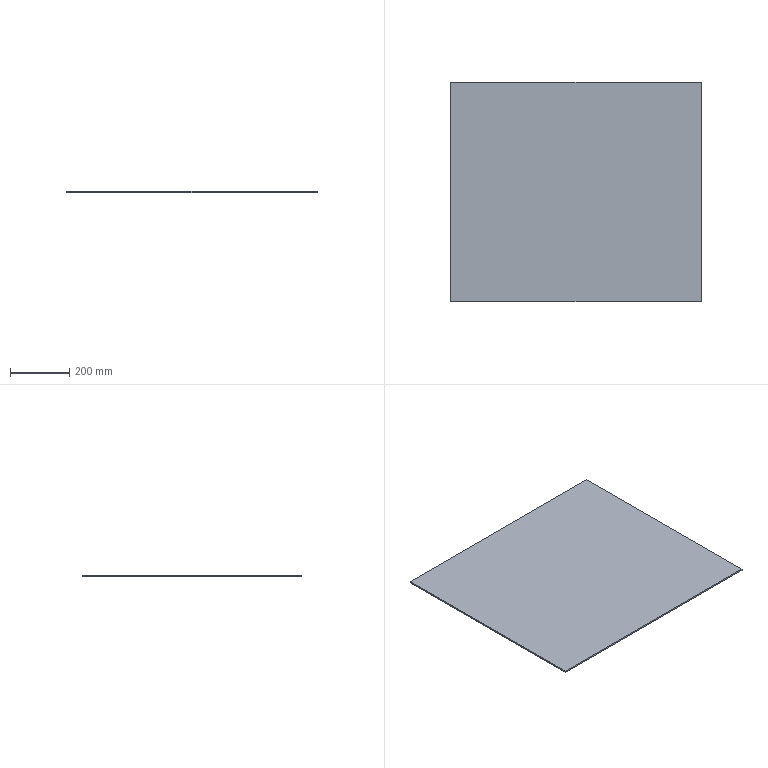Part | SolidWorks | features BaseBody 1 | 1 solid | 6 faces | box 843 x 739 x 5 mm | volume 3114885 mm3 | plane 6
STEP:
#1=CARTESIAN_POINT('',(0.,739.,5.));
#2=VERTEX_POINT('',#1);
#3=CARTESIAN_POINT('',(0.,739.,0.));
#4=VERTEX_POINT('',#3);
#5=CARTESIAN_POINT('',(0.,739.,2.5));
#6=DIRECTION('',(0.,0.,-1.));
#7=VECTOR('',#6,1000.);
#8=LINE('',#5,#7);
#9=EDGE_CURVE('',#2,#4,#8,.T.);
#10=ORIENTED_EDGE('',*,*,#9,.F.);
#11=CARTESIAN_POINT('',(0.,0.,5.));
#12=VERTEX_POINT('',#11);
#13=CARTESIAN_POINT('',(0.,369.5,5.));
#14=DIRECTION('',(0.,1.,0.));
#15=VECTOR('',#14,1000.);
#16=LINE('',#13,#15);
#17=EDGE_CURVE('',#12,#2,#16,.T.);
#18=ORIENTED_EDGE('',*,*,#17,.F.);
#19=CARTESIAN_POINT('',(0.,0.,0.));
#20=VERTEX_POINT('',#19);
#21=CARTESIAN_POINT('',(0.,0.,2.5));
#22=DIRECTION('',(0.,0.,1.));
#23=VECTOR('',#22,1000.);
#24=LINE('',#21,#23);
#25=EDGE_CURVE('',#20,#12,#24,.T.);
#26=ORIENTED_EDGE('',*,*,#25,.F.);
#27=CARTESIAN_POINT('',(0.,369.5,0.));
#28=DIRECTION('',(0.,-1.,0.));
#29=VECTOR('',#28,1000.);
#30=LINE('',#27,#29);
#31=EDGE_CURVE('',#4,#20,#30,.T.);
#32=ORIENTED_EDGE('',*,*,#31,.F.);
#33=EDGE_LOOP('',(#10,#18,#26,#32));
#34=FACE_OUTER_BOUND('',#33,.T.);
#35=CARTESIAN_POINT('',(0.,0.,0.));
#36=DIRECTION('',(-1.,0.,0.));
#37=DIRECTION('',(0.,0.,1.));
#38=AXIS2_PLACEMENT_3D('',#35,#36,#37);
#39=PLANE('',#38);
#40=ADVANCED_FACE('',(#34),#39,.F.);
#41=CARTESIAN_POINT('',(-843.,0.,0.));
#42=VERTEX_POINT('',#41);
#43=CARTESIAN_POINT('',(-421.5,0.,0.));
#44=DIRECTION('',(1.,0.,0.));
#45=VECTOR('',#44,1000.);
#46=LINE('',#43,#45);
#47=EDGE_CURVE('',#42,#20,#46,.T.);
#48=ORIENTED_EDGE('',*,*,#47,.F.);
#49=CARTESIAN_POINT('',(-843.,739.,0.));
#50=VERTEX_POINT('',#49);
#51=CARTESIAN_POINT('',(-843.,369.5,0.));
#52=DIRECTION('',(0.,-1.,0.));
#53=VECTOR('',#52,1000.);
#54=LINE('',#51,#53);
#55=EDGE_CURVE('',#50,#42,#54,.T.);
#56=ORIENTED_EDGE('',*,*,#55,.F.);
#57=CARTESIAN_POINT('',(-421.5,739.,0.));
#58=DIRECTION('',(-1.,0.,0.));
#59=VECTOR('',#58,1000.);
#60=LINE('',#57,#59);
#61=EDGE_CURVE('',#4,#50,#60,.T.);
#62=ORIENTED_EDGE('',*,*,#61,.F.);
#63=ORIENTED_EDGE('',*,*,#31,.T.);
#64=EDGE_LOOP('',(#48,#56,#62,#63));
#65=FACE_OUTER_BOUND('',#64,.T.);
#66=CARTESIAN_POINT('',(-843.,0.,0.));
#67=DIRECTION('',(0.,0.,1.));
#68=DIRECTION('',(1.,0.,0.));
#69=AXIS2_PLACEMENT_3D('',#66,#67,#68);
#70=PLANE('',#69);
#71=ADVANCED_FACE('',(#65),#70,.F.);
#72=CARTESIAN_POINT('',(-843.,739.,5.));
#73=VERTEX_POINT('',#72);
#74=CARTESIAN_POINT('',(-843.,739.,2.5));
#75=DIRECTION('',(0.,0.,-1.));
#76=VECTOR('',#75,1000.);
#77=LINE('',#74,#76);
#78=EDGE_CURVE('',#73,#50,#77,.T.);
#79=ORIENTED_EDGE('',*,*,#78,.F.);
#80=CARTESIAN_POINT('',(-421.5,739.,5.));
#81=DIRECTION('',(-1.,0.,0.));
#82=VECTOR('',#81,1000.);
#83=LINE('',#80,#82);
#84=EDGE_CURVE('',#2,#73,#83,.T.);
#85=ORIENTED_EDGE('',*,*,#84,.F.);
#86=ORIENTED_EDGE('',*,*,#9,.T.);
#87=ORIENTED_EDGE('',*,*,#61,.T.);
#88=EDGE_LOOP('',(#79,#85,#86,#87));
#89=FACE_OUTER_BOUND('',#88,.T.);
#90=CARTESIAN_POINT('',(-843.,739.,0.));
#91=DIRECTION('',(0.,-1.,0.));
#92=DIRECTION('',(1.,0.,0.));
#93=AXIS2_PLACEMENT_3D('',#90,#91,#92);
#94=PLANE('',#93);
#95=ADVANCED_FACE('',(#89),#94,.F.);
#96=CARTESIAN_POINT('',(-843.,0.,5.));
#97=VERTEX_POINT('',#96);
#98=CARTESIAN_POINT('',(-843.,369.5,5.));
#99=DIRECTION('',(0.,-1.,0.));
#100=VECTOR('',#99,1000.);
#101=LINE('',#98,#100);
#102=EDGE_CURVE('',#73,#97,#101,.T.);
#103=ORIENTED_EDGE('',*,*,#102,.T.);
#104=CARTESIAN_POINT('',(-421.5,0.,5.));
#105=DIRECTION('',(1.,0.,0.));
#106=VECTOR('',#105,1000.);
#107=LINE('',#104,#106);
#108=EDGE_CURVE('',#97,#12,#107,.T.);
#109=ORIENTED_EDGE('',*,*,#108,.T.);
#110=ORIENTED_EDGE('',*,*,#17,.T.);
#111=ORIENTED_EDGE('',*,*,#84,.T.);
#112=EDGE_LOOP('',(#103,#109,#110,#111));
#113=FACE_OUTER_BOUND('',#112,.T.);
#114=CARTESIAN_POINT('',(-843.,0.,5.));
#115=DIRECTION('',(0.,0.,1.));
#116=DIRECTION('',(1.,0.,0.));
#117=AXIS2_PLACEMENT_3D('',#114,#115,#116);
#118=PLANE('',#117);
#119=ADVANCED_FACE('',(#113),#118,.T.);
#120=ORIENTED_EDGE('',*,*,#25,.T.);
#121=ORIENTED_EDGE('',*,*,#108,.F.);
#122=CARTESIAN_POINT('',(-843.,0.,2.5));
#123=DIRECTION('',(0.,0.,1.));
#124=VECTOR('',#123,1000.);
#125=LINE('',#122,#124);
#126=EDGE_CURVE('',#42,#97,#125,.T.);
#127=ORIENTED_EDGE('',*,*,#126,.F.);
#128=ORIENTED_EDGE('',*,*,#47,.T.);
#129=EDGE_LOOP('',(#120,#121,#127,#128));
#130=FACE_OUTER_BOUND('',#129,.T.);
#131=CARTESIAN_POINT('',(0.,0.,0.));
#132=DIRECTION('',(0.,1.,0.));
#133=DIRECTION('',(-1.,0.,0.));
#134=AXIS2_PLACEMENT_3D('',#131,#132,#133);
#135=PLANE('',#134);
#136=ADVANCED_FACE('',(#130),#135,.F.);
#137=ORIENTED_EDGE('',*,*,#126,.T.);
#138=ORIENTED_EDGE('',*,*,#102,.F.);
#139=ORIENTED_EDGE('',*,*,#78,.T.);
#140=ORIENTED_EDGE('',*,*,#55,.T.);
#141=EDGE_LOOP('',(#137,#138,#139,#140));
#142=FACE_OUTER_BOUND('',#141,.T.);
#143=CARTESIAN_POINT('',(-843.,0.,5.));
#144=DIRECTION('',(1.,0.,0.));
#145=DIRECTION('',(0.,0.,-1.));
#146=AXIS2_PLACEMENT_3D('',#143,#144,#145);
#147=PLANE('',#146);
#148=ADVANCED_FACE('',(#142),#147,.F.);
#149=CLOSED_SHELL('',(#40,#71,#95,#119,#136,#148));
#150=MANIFOLD_SOLID_BREP('',#149);
#151=CARTESIAN_POINT('',(0.,0.,0.));
#152=DIRECTION('',(0.,0.,1.));
#153=DIRECTION('',(1.,0.,0.));
#154=AXIS2_PLACEMENT_3D('',#151,#152,#153);
#155=(LENGTH_UNIT()NAMED_UNIT(*)SI_UNIT(.MILLI.,.METRE.));
#156=UNCERTAINTY_MEASURE_WITH_UNIT(LENGTH_MEASURE(0.00001),#155,'','');
#157=(NAMED_UNIT(*)PLANE_ANGLE_UNIT()SI_UNIT($,.RADIAN.));
#158=(NAMED_UNIT(*)SI_UNIT($,.STERADIAN.)SOLID_ANGLE_UNIT());
#159=(GEOMETRIC_REPRESENTATION_CONTEXT(3)GLOBAL_UNCERTAINTY_ASSIGNED_CONTEXT((#156))GLOBAL_UNIT_ASSIGNED_CONTEXT((#155,#157,#158))REPRESENTATION_CONTEXT('',''));
#160=ADVANCED_BREP_SHAPE_REPRESENTATION('',(#150,#154),#159);